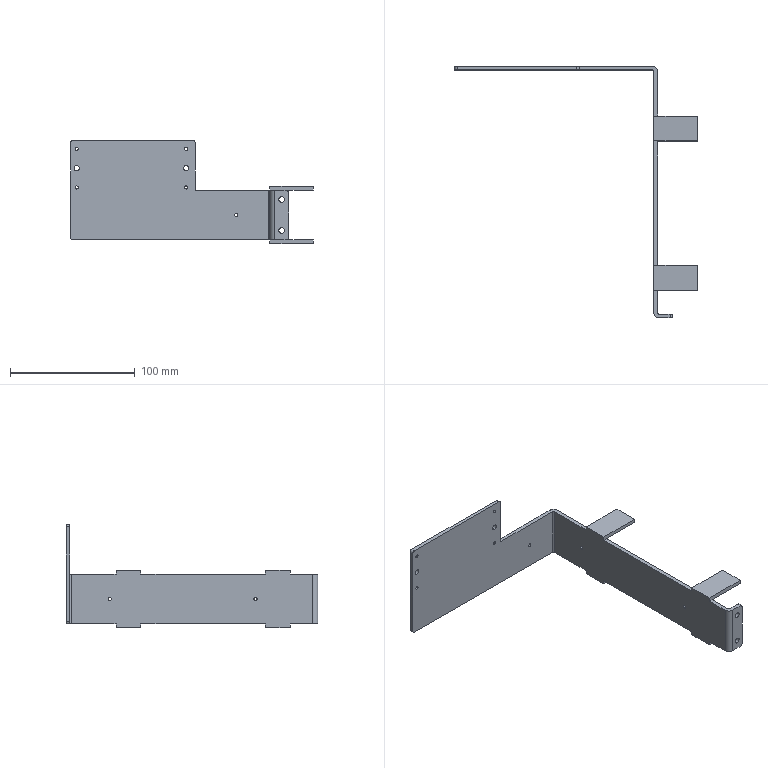Part | STEP file | 1 solid | 71 faces | box 195 x 202 x 83 mm | volume 64728 mm3 | plane 40 | cylinder 31 | commonest cylinder face diameters 2.5 x14 4 x5 4.2 x4 4.5 x4 2 x2 8 x2